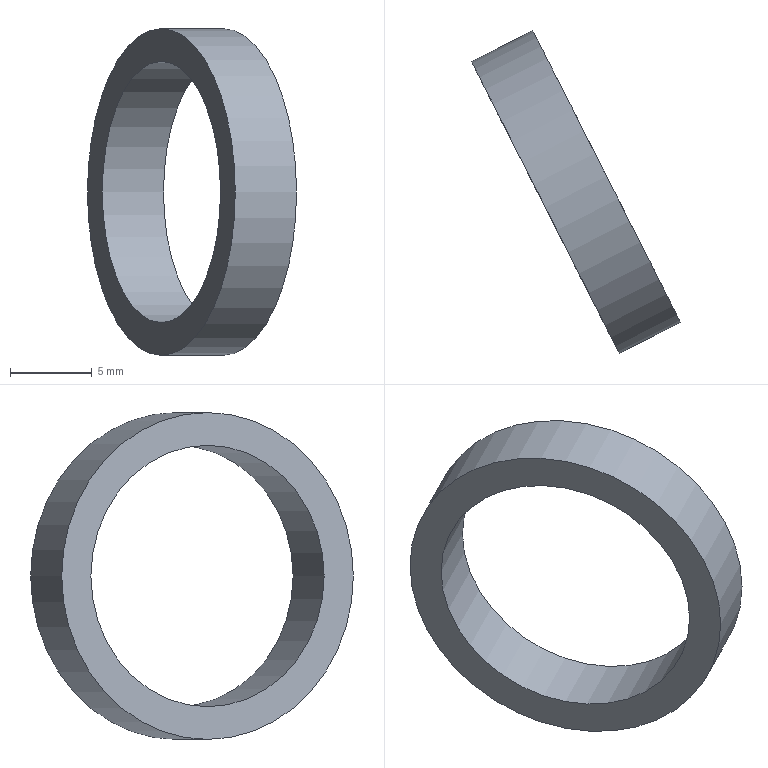Part | STEP file | solid 199 | 1 solid | 4 faces | box 12.786 x 19.739 x 20 mm | volume 475.009 mm3 | plane 2 | cylinder 2 | commonest cylinder face diameters 16 x1 20 x1